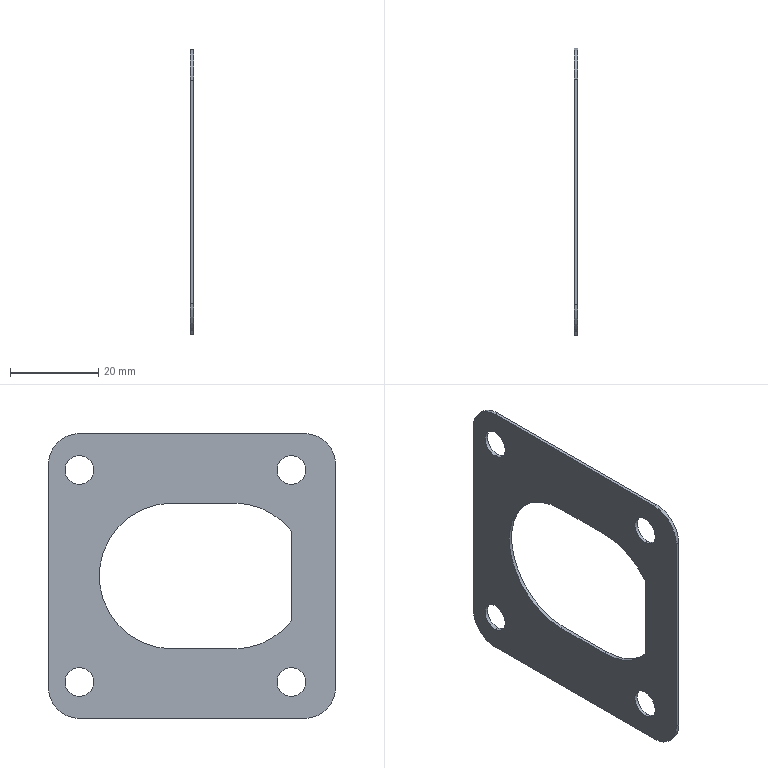Part | SolidWorks | features BaseBody 1 | 1 solid | 24 faces | box 0.8 x 65 x 64.5 mm | volume 2199 mm3 | cylinder 15 | plane 9 | commonest cylinder face diameters 6.5 x8 14 x4 33 x3
STEP:
#1=CARTESIAN_POINT('',(438.9,15.,20.75));
#2=VERTEX_POINT('',#1);
#3=CARTESIAN_POINT('',(438.9,15.,27.25));
#4=VERTEX_POINT('',#3);
#5=CARTESIAN_POINT('',(438.9,15.,24.));
#6=DIRECTION('',(1.,0.,0.));
#7=DIRECTION('',(0.,0.,-1.));
#8=AXIS2_PLACEMENT_3D('',#5,#6,#7);
#9=CIRCLE('',#8,3.25);
#10=EDGE_CURVE('',#2,#4,#9,.T.);
#11=ORIENTED_EDGE('',*,*,#10,.T.);
#12=CARTESIAN_POINT('',(438.1,15.,27.25));
#13=VERTEX_POINT('',#12);
#14=CARTESIAN_POINT('',(438.9,15.,27.25));
#15=DIRECTION('',(-1.,0.,0.));
#16=VECTOR('',#15,1000.);
#17=LINE('',#14,#16);
#18=EDGE_CURVE('',#4,#13,#17,.T.);
#19=ORIENTED_EDGE('',*,*,#18,.T.);
#20=CARTESIAN_POINT('',(438.1,15.,20.75));
#21=VERTEX_POINT('',#20);
#22=CARTESIAN_POINT('',(438.1,15.,24.));
#23=DIRECTION('',(1.,0.,0.));
#24=DIRECTION('',(0.,0.,-1.));
#25=AXIS2_PLACEMENT_3D('',#22,#23,#24);
#26=CIRCLE('',#25,3.25);
#27=EDGE_CURVE('',#21,#13,#26,.T.);
#28=ORIENTED_EDGE('',*,*,#27,.F.);
#29=CARTESIAN_POINT('',(438.9,15.,20.75));
#30=DIRECTION('',(-1.,0.,0.));
#31=VECTOR('',#30,1000.);
#32=LINE('',#29,#31);
#33=EDGE_CURVE('',#2,#21,#32,.T.);
#34=ORIENTED_EDGE('',*,*,#33,.F.);
#35=EDGE_LOOP('',(#11,#19,#28,#34));
#36=FACE_OUTER_BOUND('',#35,.T.);
#37=CARTESIAN_POINT('',(438.9,15.,24.));
#38=DIRECTION('',(-1.,0.,0.));
#39=DIRECTION('',(0.,0.,-1.));
#40=AXIS2_PLACEMENT_3D('',#37,#38,#39);
#41=CYLINDRICAL_SURFACE('',#40,3.25);
#42=ADVANCED_FACE('',(#36),#41,.F.);
#43=CARTESIAN_POINT('',(438.9,63.,20.75));
#44=VERTEX_POINT('',#43);
#45=CARTESIAN_POINT('',(438.9,63.,27.25));
#46=VERTEX_POINT('',#45);
#47=CARTESIAN_POINT('',(438.9,63.,24.));
#48=DIRECTION('',(1.,0.,0.));
#49=DIRECTION('',(0.,0.,-1.));
#50=AXIS2_PLACEMENT_3D('',#47,#48,#49);
#51=CIRCLE('',#50,3.25);
#52=EDGE_CURVE('',#44,#46,#51,.T.);
#53=ORIENTED_EDGE('',*,*,#52,.T.);
#54=CARTESIAN_POINT('',(438.1,63.,27.25));
#55=VERTEX_POINT('',#54);
#56=CARTESIAN_POINT('',(438.9,63.,27.25));
#57=DIRECTION('',(-1.,0.,0.));
#58=VECTOR('',#57,1000.);
#59=LINE('',#56,#58);
#60=EDGE_CURVE('',#46,#55,#59,.T.);
#61=ORIENTED_EDGE('',*,*,#60,.T.);
#62=CARTESIAN_POINT('',(438.1,63.,20.75));
#63=VERTEX_POINT('',#62);
#64=CARTESIAN_POINT('',(438.1,63.,24.));
#65=DIRECTION('',(1.,0.,0.));
#66=DIRECTION('',(0.,0.,-1.));
#67=AXIS2_PLACEMENT_3D('',#64,#65,#66);
#68=CIRCLE('',#67,3.25);
#69=EDGE_CURVE('',#63,#55,#68,.T.);
#70=ORIENTED_EDGE('',*,*,#69,.F.);
#71=CARTESIAN_POINT('',(438.9,63.,20.75));
#72=DIRECTION('',(-1.,0.,0.));
#73=VECTOR('',#72,1000.);
#74=LINE('',#71,#73);
#75=EDGE_CURVE('',#44,#63,#74,.T.);
#76=ORIENTED_EDGE('',*,*,#75,.F.);
#77=EDGE_LOOP('',(#53,#61,#70,#76));
#78=FACE_OUTER_BOUND('',#77,.T.);
#79=CARTESIAN_POINT('',(438.9,63.,24.));
#80=DIRECTION('',(-1.,0.,0.));
#81=DIRECTION('',(0.,0.,-1.));
#82=AXIS2_PLACEMENT_3D('',#79,#80,#81);
#83=CYLINDRICAL_SURFACE('',#82,3.25);
#84=ADVANCED_FACE('',(#78),#83,.F.);
#85=CARTESIAN_POINT('',(438.9,15.,-27.25));
#86=VERTEX_POINT('',#85);
#87=CARTESIAN_POINT('',(438.9,15.,-20.75));
#88=VERTEX_POINT('',#87);
#89=CARTESIAN_POINT('',(438.9,15.,-24.));
#90=DIRECTION('',(1.,0.,0.));
#91=DIRECTION('',(0.,0.,1.));
#92=AXIS2_PLACEMENT_3D('',#89,#90,#91);
#93=CIRCLE('',#92,3.25);
#94=EDGE_CURVE('',#86,#88,#93,.T.);
#95=ORIENTED_EDGE('',*,*,#94,.T.);
#96=CARTESIAN_POINT('',(438.1,15.,-20.75));
#97=VERTEX_POINT('',#96);
#98=CARTESIAN_POINT('',(438.9,15.,-20.75));
#99=DIRECTION('',(-1.,0.,0.));
#100=VECTOR('',#99,1000.);
#101=LINE('',#98,#100);
#102=EDGE_CURVE('',#88,#97,#101,.T.);
#103=ORIENTED_EDGE('',*,*,#102,.T.);
#104=CARTESIAN_POINT('',(438.1,15.,-27.25));
#105=VERTEX_POINT('',#104);
#106=CARTESIAN_POINT('',(438.1,15.,-24.));
#107=DIRECTION('',(1.,0.,0.));
#108=DIRECTION('',(0.,0.,1.));
#109=AXIS2_PLACEMENT_3D('',#106,#107,#108);
#110=CIRCLE('',#109,3.25);
#111=EDGE_CURVE('',#105,#97,#110,.T.);
#112=ORIENTED_EDGE('',*,*,#111,.F.);
#113=CARTESIAN_POINT('',(438.9,15.,-27.25));
#114=DIRECTION('',(-1.,0.,0.));
#115=VECTOR('',#114,1000.);
#116=LINE('',#113,#115);
#117=EDGE_CURVE('',#86,#105,#116,.T.);
#118=ORIENTED_EDGE('',*,*,#117,.F.);
#119=EDGE_LOOP('',(#95,#103,#112,#118));
#120=FACE_OUTER_BOUND('',#119,.T.);
#121=CARTESIAN_POINT('',(438.9,15.,-24.));
#122=DIRECTION('',(-1.,0.,0.));
#123=DIRECTION('',(0.,0.,-1.));
#124=AXIS2_PLACEMENT_3D('',#121,#122,#123);
#125=CYLINDRICAL_SURFACE('',#124,3.25);
#126=ADVANCED_FACE('',(#120),#125,.F.);
#127=CARTESIAN_POINT('',(438.9,63.,-27.25));
#128=VERTEX_POINT('',#127);
#129=CARTESIAN_POINT('',(438.9,63.,-20.75));
#130=VERTEX_POINT('',#129);
#131=CARTESIAN_POINT('',(438.9,63.,-24.));
#132=DIRECTION('',(1.,0.,0.));
#133=DIRECTION('',(0.,0.,1.));
#134=AXIS2_PLACEMENT_3D('',#131,#132,#133);
#135=CIRCLE('',#134,3.25);
#136=EDGE_CURVE('',#128,#130,#135,.T.);
#137=ORIENTED_EDGE('',*,*,#136,.T.);
#138=CARTESIAN_POINT('',(438.1,63.,-20.75));
#139=VERTEX_POINT('',#138);
#140=CARTESIAN_POINT('',(438.9,63.,-20.75));
#141=DIRECTION('',(-1.,0.,0.));
#142=VECTOR('',#141,1000.);
#143=LINE('',#140,#142);
#144=EDGE_CURVE('',#130,#139,#143,.T.);
#145=ORIENTED_EDGE('',*,*,#144,.T.);
#146=CARTESIAN_POINT('',(438.1,63.,-27.25));
#147=VERTEX_POINT('',#146);
#148=CARTESIAN_POINT('',(438.1,63.,-24.));
#149=DIRECTION('',(1.,0.,0.));
#150=DIRECTION('',(0.,0.,1.));
#151=AXIS2_PLACEMENT_3D('',#148,#149,#150);
#152=CIRCLE('',#151,3.25);
#153=EDGE_CURVE('',#147,#139,#152,.T.);
#154=ORIENTED_EDGE('',*,*,#153,.F.);
#155=CARTESIAN_POINT('',(438.9,63.,-27.25));
#156=DIRECTION('',(-1.,0.,0.));
#157=VECTOR('',#156,1000.);
#158=LINE('',#155,#157);
#159=EDGE_CURVE('',#128,#147,#158,.T.);
#160=ORIENTED_EDGE('',*,*,#159,.F.);
#161=EDGE_LOOP('',(#137,#145,#154,#160));
#162=FACE_OUTER_BOUND('',#161,.T.);
#163=CARTESIAN_POINT('',(438.9,63.,-24.));
#164=DIRECTION('',(-1.,0.,0.));
#165=DIRECTION('',(0.,0.,-1.));
#166=AXIS2_PLACEMENT_3D('',#163,#164,#165);
#167=CYLINDRICAL_SURFACE('',#166,3.25);
#168=ADVANCED_FACE('',(#162),#167,.F.);
#169=ORIENTED_EDGE('',*,*,#52,.F.);
#170=CARTESIAN_POINT('',(438.9,63.,24.));
#171=DIRECTION('',(1.,0.,0.));
#172=DIRECTION('',(0.,0.,-1.));
#173=AXIS2_PLACEMENT_3D('',#170,#171,#172);
#174=CIRCLE('',#173,3.25);
#175=EDGE_CURVE('',#46,#44,#174,.T.);
#176=ORIENTED_EDGE('',*,*,#175,.F.);
#177=EDGE_LOOP('',(#169,#176));
#178=FACE_BOUND('',#177,.T.);
#179=ORIENTED_EDGE('',*,*,#94,.F.);
#180=CARTESIAN_POINT('',(438.9,15.,-24.));
#181=DIRECTION('',(1.,0.,0.));
#182=DIRECTION('',(0.,0.,1.));
#183=AXIS2_PLACEMENT_3D('',#180,#181,#182);
#184=CIRCLE('',#183,3.25);
#185=EDGE_CURVE('',#88,#86,#184,.T.);
#186=ORIENTED_EDGE('',*,*,#185,.F.);
#187=EDGE_LOOP('',(#179,#186));
#188=FACE_BOUND('',#187,.T.);
#189=CARTESIAN_POINT('',(438.9,5.,-25.25));
#190=VERTEX_POINT('',#189);
#191=CARTESIAN_POINT('',(438.9,12.,-32.25));
#192=VERTEX_POINT('',#191);
#193=CARTESIAN_POINT('',(438.9,12.,-25.25));
#194=DIRECTION('',(1.,0.,0.));
#195=DIRECTION('',(0.,0.,1.));
#196=AXIS2_PLACEMENT_3D('',#193,#194,#195);
#197=CIRCLE('',#196,7.);
#198=EDGE_CURVE('',#190,#192,#197,.T.);
#199=ORIENTED_EDGE('',*,*,#198,.T.);
#200=CARTESIAN_POINT('',(438.9,63.,-32.25));
#201=VERTEX_POINT('',#200);
#202=CARTESIAN_POINT('',(438.9,12.,-32.25));
#203=DIRECTION('',(0.,1.,0.));
#204=VECTOR('',#203,1000.);
#205=LINE('',#202,#204);
#206=EDGE_CURVE('',#192,#201,#205,.T.);
#207=ORIENTED_EDGE('',*,*,#206,.T.);
#208=CARTESIAN_POINT('',(438.9,70.,-25.25));
#209=VERTEX_POINT('',#208);
#210=CARTESIAN_POINT('',(438.9,63.,-25.25));
#211=DIRECTION('',(1.,0.,0.));
#212=DIRECTION('',(0.,0.,1.));
#213=AXIS2_PLACEMENT_3D('',#210,#211,#212);
#214=CIRCLE('',#213,7.);
#215=EDGE_CURVE('',#201,#209,#214,.T.);
#216=ORIENTED_EDGE('',*,*,#215,.T.);
#217=CARTESIAN_POINT('',(438.9,70.,25.25));
#218=VERTEX_POINT('',#217);
#219=CARTESIAN_POINT('',(438.9,70.,-25.25));
#220=DIRECTION('',(0.,0.,1.));
#221=VECTOR('',#220,1000.);
#222=LINE('',#219,#221);
#223=EDGE_CURVE('',#209,#218,#222,.T.);
#224=ORIENTED_EDGE('',*,*,#223,.T.);
#225=CARTESIAN_POINT('',(438.9,63.,32.25));
#226=VERTEX_POINT('',#225);
#227=CARTESIAN_POINT('',(438.9,63.,25.25));
#228=DIRECTION('',(1.,0.,0.));
#229=DIRECTION('',(0.,0.,1.));
#230=AXIS2_PLACEMENT_3D('',#227,#228,#229);
#231=CIRCLE('',#230,7.);
#232=EDGE_CURVE('',#218,#226,#231,.T.);
#233=ORIENTED_EDGE('',*,*,#232,.T.);
#234=CARTESIAN_POINT('',(438.9,12.,32.25));
#235=VERTEX_POINT('',#234);
#236=CARTESIAN_POINT('',(438.9,12.,32.25));
#237=DIRECTION('',(0.,-1.,0.));
#238=VECTOR('',#237,1000.);
#239=LINE('',#236,#238);
#240=EDGE_CURVE('',#226,#235,#239,.T.);
#241=ORIENTED_EDGE('',*,*,#240,.T.);
#242=CARTESIAN_POINT('',(438.9,5.,25.25));
#243=VERTEX_POINT('',#242);
#244=CARTESIAN_POINT('',(438.9,12.,25.25));
#245=DIRECTION('',(1.,0.,0.));
#246=DIRECTION('',(0.,0.,-1.));
#247=AXIS2_PLACEMENT_3D('',#244,#245,#246);
#248=CIRCLE('',#247,7.);
#249=EDGE_CURVE('',#235,#243,#248,.T.);
#250=ORIENTED_EDGE('',*,*,#249,.T.);
#251=CARTESIAN_POINT('',(438.9,5.,-25.25));
#252=DIRECTION('',(0.,0.,-1.));
#253=VECTOR('',#252,1000.);
#254=LINE('',#251,#253);
#255=EDGE_CURVE('',#243,#190,#254,.T.);
#256=ORIENTED_EDGE('',*,*,#255,.T.);
#257=EDGE_LOOP('',(#199,#207,#216,#224,#233,#241,#250,#256));
#258=FACE_OUTER_BOUND('',#257,.T.);
#259=ORIENTED_EDGE('',*,*,#136,.F.);
#260=CARTESIAN_POINT('',(438.9,63.,-24.));
#261=DIRECTION('',(1.,0.,0.));
#262=DIRECTION('',(0.,0.,1.));
#263=AXIS2_PLACEMENT_3D('',#260,#261,#262);
#264=CIRCLE('',#263,3.25);
#265=EDGE_CURVE('',#130,#128,#264,.T.);
#266=ORIENTED_EDGE('',*,*,#265,.F.);
#267=EDGE_LOOP('',(#259,#266));
#268=FACE_BOUND('',#267,.T.);
#269=CARTESIAN_POINT('',(438.9,15.,10.161));
#270=VERTEX_POINT('',#269);
#271=CARTESIAN_POINT('',(438.9,15.,-10.161));
#272=VERTEX_POINT('',#271);
#273=CARTESIAN_POINT('',(438.9,15.,-10.161));
#274=DIRECTION('',(0.,0.,-1.));
#275=VECTOR('',#274,1000.);
#276=LINE('',#273,#275);
#277=EDGE_CURVE('',#270,#272,#276,.T.);
#278=ORIENTED_EDGE('',*,*,#277,.F.);
#279=CARTESIAN_POINT('',(438.9,28.,16.5));
#280=VERTEX_POINT('',#279);
#281=CARTESIAN_POINT('',(438.9,28.,0.));
#282=DIRECTION('',(1.,0.,0.));
#283=DIRECTION('',(0.,0.,1.));
#284=AXIS2_PLACEMENT_3D('',#281,#282,#283);
#285=CIRCLE('',#284,16.5);
#286=EDGE_CURVE('',#280,#270,#285,.T.);
#287=ORIENTED_EDGE('',*,*,#286,.F.);
#288=CARTESIAN_POINT('',(438.9,42.,16.5));
#289=VERTEX_POINT('',#288);
#290=CARTESIAN_POINT('',(438.9,28.,16.5));
#291=DIRECTION('',(0.,-1.,0.));
#292=VECTOR('',#291,1000.);
#293=LINE('',#290,#292);
#294=EDGE_CURVE('',#289,#280,#293,.T.);
#295=ORIENTED_EDGE('',*,*,#294,.F.);
#296=CARTESIAN_POINT('',(438.9,42.,-16.5));
#297=VERTEX_POINT('',#296);
#298=CARTESIAN_POINT('',(438.9,42.,0.));
#299=DIRECTION('',(1.,0.,0.));
#300=DIRECTION('',(0.,0.,1.));
#301=AXIS2_PLACEMENT_3D('',#298,#299,#300);
#302=CIRCLE('',#301,16.5);
#303=EDGE_CURVE('',#297,#289,#302,.T.);
#304=ORIENTED_EDGE('',*,*,#303,.F.);
#305=CARTESIAN_POINT('',(438.9,28.,-16.5));
#306=VERTEX_POINT('',#305);
#307=CARTESIAN_POINT('',(438.9,42.,-16.5));
#308=DIRECTION('',(0.,1.,0.));
#309=VECTOR('',#308,1000.);
#310=LINE('',#307,#309);
#311=EDGE_CURVE('',#306,#297,#310,.T.);
#312=ORIENTED_EDGE('',*,*,#311,.F.);
#313=CARTESIAN_POINT('',(438.9,28.,0.));
#314=DIRECTION('',(1.,0.,0.));
#315=DIRECTION('',(0.,0.,1.));
#316=AXIS2_PLACEMENT_3D('',#313,#314,#315);
#317=CIRCLE('',#316,16.5);
#318=EDGE_CURVE('',#272,#306,#317,.T.);
#319=ORIENTED_EDGE('',*,*,#318,.F.);
#320=EDGE_LOOP('',(#278,#287,#295,#304,#312,#319));
#321=FACE_BOUND('',#320,.T.);
#322=ORIENTED_EDGE('',*,*,#10,.F.);
#323=CARTESIAN_POINT('',(438.9,15.,24.));
#324=DIRECTION('',(1.,0.,0.));
#325=DIRECTION('',(0.,0.,-1.));
#326=AXIS2_PLACEMENT_3D('',#323,#324,#325);
#327=CIRCLE('',#326,3.25);
#328=EDGE_CURVE('',#4,#2,#327,.T.);
#329=ORIENTED_EDGE('',*,*,#328,.F.);
#330=EDGE_LOOP('',(#322,#329));
#331=FACE_BOUND('',#330,.T.);
#332=CARTESIAN_POINT('',(438.9,12.,-25.25));
#333=DIRECTION('',(1.,0.,0.));
#334=DIRECTION('',(0.,0.,1.));
#335=AXIS2_PLACEMENT_3D('',#332,#333,#334);
#336=PLANE('',#335);
#337=ADVANCED_FACE('',(#178,#188,#258,#268,#321,#331),#336,.T.);
#338=ORIENTED_EDGE('',*,*,#69,.T.);
#339=CARTESIAN_POINT('',(438.1,63.,24.));
#340=DIRECTION('',(1.,0.,0.));
#341=DIRECTION('',(0.,0.,-1.));
#342=AXIS2_PLACEMENT_3D('',#339,#340,#341);
#343=CIRCLE('',#342,3.25);
#344=EDGE_CURVE('',#55,#63,#343,.T.);
#345=ORIENTED_EDGE('',*,*,#344,.T.);
#346=EDGE_LOOP('',(#338,#345));
#347=FACE_BOUND('',#346,.T.);
#348=ORIENTED_EDGE('',*,*,#111,.T.);
#349=CARTESIAN_POINT('',(438.1,15.,-24.));
#350=DIRECTION('',(1.,0.,0.));
#351=DIRECTION('',(0.,0.,1.));
#352=AXIS2_PLACEMENT_3D('',#349,#350,#351);
#353=CIRCLE('',#352,3.25);
#354=EDGE_CURVE('',#97,#105,#353,.T.);
#355=ORIENTED_EDGE('',*,*,#354,.T.);
#356=EDGE_LOOP('',(#348,#355));
#357=FACE_BOUND('',#356,.T.);
#358=CARTESIAN_POINT('',(438.1,5.,-25.25));
#359=VERTEX_POINT('',#358);
#360=CARTESIAN_POINT('',(438.1,12.,-32.25));
#361=VERTEX_POINT('',#360);
#362=CARTESIAN_POINT('',(438.1,12.,-25.25));
#363=DIRECTION('',(1.,0.,0.));
#364=DIRECTION('',(0.,0.,1.));
#365=AXIS2_PLACEMENT_3D('',#362,#363,#364);
#366=CIRCLE('',#365,7.);
#367=EDGE_CURVE('',#359,#361,#366,.T.);
#368=ORIENTED_EDGE('',*,*,#367,.F.);
#369=CARTESIAN_POINT('',(438.1,5.,25.25));
#370=VERTEX_POINT('',#369);
#371=CARTESIAN_POINT('',(438.1,5.,-25.25));
#372=DIRECTION('',(0.,0.,-1.));
#373=VECTOR('',#372,1000.);
#374=LINE('',#371,#373);
#375=EDGE_CURVE('',#370,#359,#374,.T.);
#376=ORIENTED_EDGE('',*,*,#375,.F.);
#377=CARTESIAN_POINT('',(438.1,12.,32.25));
#378=VERTEX_POINT('',#377);
#379=CARTESIAN_POINT('',(438.1,12.,25.25));
#380=DIRECTION('',(1.,0.,0.));
#381=DIRECTION('',(0.,0.,-1.));
#382=AXIS2_PLACEMENT_3D('',#379,#380,#381);
#383=CIRCLE('',#382,7.);
#384=EDGE_CURVE('',#378,#370,#383,.T.);
#385=ORIENTED_EDGE('',*,*,#384,.F.);
#386=CARTESIAN_POINT('',(438.1,63.,32.25));
#387=VERTEX_POINT('',#386);
#388=CARTESIAN_POINT('',(438.1,12.,32.25));
#389=DIRECTION('',(0.,-1.,0.));
#390=VECTOR('',#389,1000.);
#391=LINE('',#388,#390);
#392=EDGE_CURVE('',#387,#378,#391,.T.);
#393=ORIENTED_EDGE('',*,*,#392,.F.);
#394=CARTESIAN_POINT('',(438.1,70.,25.25));
#395=VERTEX_POINT('',#394);
#396=CARTESIAN_POINT('',(438.1,63.,25.25));
#397=DIRECTION('',(1.,0.,0.));
#398=DIRECTION('',(0.,0.,1.));
#399=AXIS2_PLACEMENT_3D('',#396,#397,#398);
#400=CIRCLE('',#399,7.);
#401=EDGE_CURVE('',#395,#387,#400,.T.);
#402=ORIENTED_EDGE('',*,*,#401,.F.);
#403=CARTESIAN_POINT('',(438.1,70.,-25.25));
#404=VERTEX_POINT('',#403);
#405=CARTESIAN_POINT('',(438.1,70.,-25.25));
#406=DIRECTION('',(0.,0.,1.));
#407=VECTOR('',#406,1000.);
#408=LINE('',#405,#407);
#409=EDGE_CURVE('',#404,#395,#408,.T.);
#410=ORIENTED_EDGE('',*,*,#409,.F.);
#411=CARTESIAN_POINT('',(438.1,63.,-32.25));
#412=VERTEX_POINT('',#411);
#413=CARTESIAN_POINT('',(438.1,63.,-25.25));
#414=DIRECTION('',(1.,0.,0.));
#415=DIRECTION('',(0.,0.,1.));
#416=AXIS2_PLACEMENT_3D('',#413,#414,#415);
#417=CIRCLE('',#416,7.);
#418=EDGE_CURVE('',#412,#404,#417,.T.);
#419=ORIENTED_EDGE('',*,*,#418,.F.);
#420=CARTESIAN_POINT('',(438.1,12.,-32.25));
#421=DIRECTION('',(0.,1.,0.));
#422=VECTOR('',#421,1000.);
#423=LINE('',#420,#422);
#424=EDGE_CURVE('',#361,#412,#423,.T.);
#425=ORIENTED_EDGE('',*,*,#424,.F.);
#426=EDGE_LOOP('',(#368,#376,#385,#393,#402,#410,#419,#425));
#427=FACE_OUTER_BOUND('',#426,.T.);
#428=ORIENTED_EDGE('',*,*,#153,.T.);
#429=CARTESIAN_POINT('',(438.1,63.,-24.));
#430=DIRECTION('',(1.,0.,0.));
#431=DIRECTION('',(0.,0.,1.));
#432=AXIS2_PLACEMENT_3D('',#429,#430,#431);
#433=CIRCLE('',#432,3.25);
#434=EDGE_CURVE('',#139,#147,#433,.T.);
#435=ORIENTED_EDGE('',*,*,#434,.T.);
#436=EDGE_LOOP('',(#428,#435));
#437=FACE_BOUND('',#436,.T.);
#438=CARTESIAN_POINT('',(438.1,28.,16.5));
#439=VERTEX_POINT('',#438);
#440=CARTESIAN_POINT('',(438.1,15.,10.161));
#441=VERTEX_POINT('',#440);
#442=CARTESIAN_POINT('',(438.1,28.,0.));
#443=DIRECTION('',(1.,0.,0.));
#444=DIRECTION('',(0.,0.,1.));
#445=AXIS2_PLACEMENT_3D('',#442,#443,#444);
#446=CIRCLE('',#445,16.5);
#447=EDGE_CURVE('',#439,#441,#446,.T.);
#448=ORIENTED_EDGE('',*,*,#447,.T.);
#449=CARTESIAN_POINT('',(438.1,15.,-10.161));
#450=VERTEX_POINT('',#449);
#451=CARTESIAN_POINT('',(438.1,15.,-10.161));
#452=DIRECTION('',(0.,0.,-1.));
#453=VECTOR('',#452,1000.);
#454=LINE('',#451,#453);
#455=EDGE_CURVE('',#441,#450,#454,.T.);
#456=ORIENTED_EDGE('',*,*,#455,.T.);
#457=CARTESIAN_POINT('',(438.1,28.,-16.5));
#458=VERTEX_POINT('',#457);
#459=CARTESIAN_POINT('',(438.1,28.,0.));
#460=DIRECTION('',(1.,0.,0.));
#461=DIRECTION('',(0.,0.,1.));
#462=AXIS2_PLACEMENT_3D('',#459,#460,#461);
#463=CIRCLE('',#462,16.5);
#464=EDGE_CURVE('',#450,#458,#463,.T.);
#465=ORIENTED_EDGE('',*,*,#464,.T.);
#466=CARTESIAN_POINT('',(438.1,42.,-16.5));
#467=VERTEX_POINT('',#466);
#468=CARTESIAN_POINT('',(438.1,42.,-16.5));
#469=DIRECTION('',(0.,1.,0.));
#470=VECTOR('',#469,1000.);
#471=LINE('',#468,#470);
#472=EDGE_CURVE('',#458,#467,#471,.T.);
#473=ORIENTED_EDGE('',*,*,#472,.T.);
#474=CARTESIAN_POINT('',(438.1,42.,16.5));
#475=VERTEX_POINT('',#474);
#476=CARTESIAN_POINT('',(438.1,42.,0.));
#477=DIRECTION('',(1.,0.,0.));
#478=DIRECTION('',(0.,0.,1.));
#479=AXIS2_PLACEMENT_3D('',#476,#477,#478);
#480=CIRCLE('',#479,16.5);
#481=EDGE_CURVE('',#467,#475,#480,.T.);
#482=ORIENTED_EDGE('',*,*,#481,.T.);
#483=CARTESIAN_POINT('',(438.1,28.,16.5));
#484=DIRECTION('',(0.,-1.,0.));
#485=VECTOR('',#484,1000.);
#486=LINE('',#483,#485);
#487=EDGE_CURVE('',#475,#439,#486,.T.);
#488=ORIENTED_EDGE('',*,*,#487,.T.);
#489=EDGE_LOOP('',(#448,#456,#465,#473,#482,#488));
#490=FACE_BOUND('',#489,.T.);
#491=ORIENTED_EDGE('',*,*,#27,.T.);
#492=CARTESIAN_POINT('',(438.1,15.,24.));
#493=DIRECTION('',(1.,0.,0.));
#494=DIRECTION('',(0.,0.,-1.));
#495=AXIS2_PLACEMENT_3D('',#492,#493,#494);
#496=CIRCLE('',#495,3.25);
#497=EDGE_CURVE('',#13,#21,#496,.T.);
#498=ORIENTED_EDGE('',*,*,#497,.T.);
#499=EDGE_LOOP('',(#491,#498));
#500=FACE_BOUND('',#499,.T.);
#501=CARTESIAN_POINT('',(438.1,12.,-25.25));
#502=DIRECTION('',(1.,0.,0.));
#503=DIRECTION('',(0.,0.,1.));
#504=AXIS2_PLACEMENT_3D('',#501,#502,#503);
#505=PLANE('',#504);
#506=ADVANCED_FACE('',(#347,#357,#427,#437,#490,#500),#505,.F.);
#507=ORIENTED_EDGE('',*,*,#367,.T.);
#508=CARTESIAN_POINT('',(438.9,12.,-32.25));
#509=DIRECTION('',(-1.,0.,0.));
#510=VECTOR('',#509,1000.);
#511=LINE('',#508,#510);
#512=EDGE_CURVE('',#192,#361,#511,.T.);
#513=ORIENTED_EDGE('',*,*,#512,.F.);
#514=ORIENTED_EDGE('',*,*,#198,.F.);
#515=CARTESIAN_POINT('',(438.9,5.,-25.25));
#516=DIRECTION('',(-1.,0.,0.));
#517=VECTOR('',#516,1000.);
#518=LINE('',#515,#517);
#519=EDGE_CURVE('',#190,#359,#518,.T.);
#520=ORIENTED_EDGE('',*,*,#519,.T.);
#521=EDGE_LOOP('',(#507,#513,#514,#520));
#522=FACE_OUTER_BOUND('',#521,.T.);
#523=CARTESIAN_POINT('',(438.9,12.,-25.25));
#524=DIRECTION('',(-1.,0.,0.));
#525=DIRECTION('',(0.,0.,-1.));
#526=AXIS2_PLACEMENT_3D('',#523,#524,#525);
#527=CYLINDRICAL_SURFACE('',#526,7.);
#528=ADVANCED_FACE('',(#522),#527,.T.);
#529=ORIENTED_EDGE('',*,*,#424,.T.);
#530=CARTESIAN_POINT('',(438.9,63.,-32.25));
#531=DIRECTION('',(-1.,0.,0.));
#532=VECTOR('',#531,1000.);
#533=LINE('',#530,#532);
#534=EDGE_CURVE('',#201,#412,#533,.T.);
#535=ORIENTED_EDGE('',*,*,#534,.F.);
#536=ORIENTED_EDGE('',*,*,#206,.F.);
#537=ORIENTED_EDGE('',*,*,#512,.T.);
#538=EDGE_LOOP('',(#529,#535,#536,#537));
#539=FACE_OUTER_BOUND('',#538,.T.);
#540=CARTESIAN_POINT('',(438.9,12.,-32.25));
#541=DIRECTION('',(0.,0.,1.));
#542=DIRECTION('',(-1.,0.,0.));
#543=AXIS2_PLACEMENT_3D('',#540,#541,#542);
#544=PLANE('',#543);
#545=ADVANCED_FACE('',(#539),#544,.F.);
#546=ORIENTED_EDGE('',*,*,#418,.T.);
#547=CARTESIAN_POINT('',(438.9,70.,-25.25));
#548=DIRECTION('',(-1.,0.,0.));
#549=VECTOR('',#548,1000.);
#550=LINE('',#547,#549);
#551=EDGE_CURVE('',#209,#404,#550,.T.);
#552=ORIENTED_EDGE('',*,*,#551,.F.);
#553=ORIENTED_EDGE('',*,*,#215,.F.);
#554=ORIENTED_EDGE('',*,*,#534,.T.);
#555=EDGE_LOOP('',(#546,#552,#553,#554));
#556=FACE_OUTER_BOUND('',#555,.T.);
#557=CARTESIAN_POINT('',(438.9,63.,-25.25));
#558=DIRECTION('',(-1.,0.,0.));
#559=DIRECTION('',(0.,0.,-1.));
#560=AXIS2_PLACEMENT_3D('',#557,#558,#559);
#561=CYLINDRICAL_SURFACE('',#560,7.);
#562=ADVANCED_FACE('',(#556),#561,.T.);
#563=ORIENTED_EDGE('',*,*,#409,.T.);
#564=CARTESIAN_POINT('',(438.9,70.,25.25));
#565=DIRECTION('',(-1.,0.,0.));
#566=VECTOR('',#565,1000.);
#567=LINE('',#564,#566);
#568=EDGE_CURVE('',#218,#395,#567,.T.);
#569=ORIENTED_EDGE('',*,*,#568,.F.);
#570=ORIENTED_EDGE('',*,*,#223,.F.);
#571=ORIENTED_EDGE('',*,*,#551,.T.);
#572=EDGE_LOOP('',(#563,#569,#570,#571));
#573=FACE_OUTER_BOUND('',#572,.T.);
#574=CARTESIAN_POINT('',(438.9,70.,-25.25));
#575=DIRECTION('',(0.,-1.,0.));
#576=DIRECTION('',(0.,0.,-1.));
#577=AXIS2_PLACEMENT_3D('',#574,#575,#576);
#578=PLANE('',#577);
#579=ADVANCED_FACE('',(#573),#578,.F.);
#580=ORIENTED_EDGE('',*,*,#401,.T.);
#581=CARTESIAN_POINT('',(438.9,63.,32.25));
#582=DIRECTION('',(-1.,0.,0.));
#583=VECTOR('',#582,1000.);
#584=LINE('',#581,#583);
#585=EDGE_CURVE('',#226,#387,#584,.T.);
#586=ORIENTED_EDGE('',*,*,#585,.F.);
#587=ORIENTED_EDGE('',*,*,#232,.F.);
#588=ORIENTED_EDGE('',*,*,#568,.T.);
#589=EDGE_LOOP('',(#580,#586,#587,#588));
#590=FACE_OUTER_BOUND('',#589,.T.);
#591=CARTESIAN_POINT('',(438.9,63.,25.25));
#592=DIRECTION('',(-1.,0.,0.));
#593=DIRECTION('',(0.,0.,-1.));
#594=AXIS2_PLACEMENT_3D('',#591,#592,#593);
#595=CYLINDRICAL_SURFACE('',#594,7.);
#596=ADVANCED_FACE('',(#590),#595,.T.);
#597=ORIENTED_EDGE('',*,*,#392,.T.);
#598=CARTESIAN_POINT('',(438.9,12.,32.25));
#599=DIRECTION('',(-1.,0.,0.));
#600=VECTOR('',#599,1000.);
#601=LINE('',#598,#600);
#602=EDGE_CURVE('',#235,#378,#601,.T.);
#603=ORIENTED_EDGE('',*,*,#602,.F.);
#604=ORIENTED_EDGE('',*,*,#240,.F.);
#605=ORIENTED_EDGE('',*,*,#585,.T.);
#606=EDGE_LOOP('',(#597,#603,#604,#605));
#607=FACE_OUTER_BOUND('',#606,.T.);
#608=CARTESIAN_POINT('',(438.9,12.,32.25));
#609=DIRECTION('',(0.,0.,-1.));
#610=DIRECTION('',(0.,1.,0.));
#611=AXIS2_PLACEMENT_3D('',#608,#609,#610);
#612=PLANE('',#611);
#613=ADVANCED_FACE('',(#607),#612,.F.);
#614=ORIENTED_EDGE('',*,*,#384,.T.);
#615=CARTESIAN_POINT('',(438.9,5.,25.25));
#616=DIRECTION('',(-1.,0.,0.));
#617=VECTOR('',#616,1000.);
#618=LINE('',#615,#617);
#619=EDGE_CURVE('',#243,#370,#618,.T.);
#620=ORIENTED_EDGE('',*,*,#619,.F.);
#621=ORIENTED_EDGE('',*,*,#249,.F.);
#622=ORIENTED_EDGE('',*,*,#602,.T.);
#623=EDGE_LOOP('',(#614,#620,#621,#622));
#624=FACE_OUTER_BOUND('',#623,.T.);
#625=CARTESIAN_POINT('',(438.9,12.,25.25));
#626=DIRECTION('',(-1.,0.,0.));
#627=DIRECTION('',(0.,0.,-1.));
#628=AXIS2_PLACEMENT_3D('',#625,#626,#627);
#629=CYLINDRICAL_SURFACE('',#628,7.);
#630=ADVANCED_FACE('',(#624),#629,.T.);
#631=ORIENTED_EDGE('',*,*,#375,.T.);
#632=ORIENTED_EDGE('',*,*,#519,.F.);
#633=ORIENTED_EDGE('',*,*,#255,.F.);
#634=ORIENTED_EDGE('',*,*,#619,.T.);
#635=EDGE_LOOP('',(#631,#632,#633,#634));
#636=FACE_OUTER_BOUND('',#635,.T.);
#637=CARTESIAN_POINT('',(438.9,5.,-25.25));
#638=DIRECTION('',(0.,1.,0.));
#639=DIRECTION('',(0.,0.,1.));
#640=AXIS2_PLACEMENT_3D('',#637,#638,#639);
#641=PLANE('',#640);
#642=ADVANCED_FACE('',(#636),#641,.F.);
#643=ORIENTED_EDGE('',*,*,#144,.F.);
#644=ORIENTED_EDGE('',*,*,#265,.T.);
#645=ORIENTED_EDGE('',*,*,#159,.T.);
#646=ORIENTED_EDGE('',*,*,#434,.F.);
#647=EDGE_LOOP('',(#643,#644,#645,#646));
#648=FACE_OUTER_BOUND('',#647,.T.);
#649=CARTESIAN_POINT('',(438.9,63.,-24.));
#650=DIRECTION('',(-1.,0.,0.));
#651=DIRECTION('',(0.,0.,-1.));
#652=AXIS2_PLACEMENT_3D('',#649,#650,#651);
#653=CYLINDRICAL_SURFACE('',#652,3.25);
#654=ADVANCED_FACE('',(#648),#653,.F.);
#655=ORIENTED_EDGE('',*,*,#102,.F.);
#656=ORIENTED_EDGE('',*,*,#185,.T.);
#657=ORIENTED_EDGE('',*,*,#117,.T.);
#658=ORIENTED_EDGE('',*,*,#354,.F.);
#659=EDGE_LOOP('',(#655,#656,#657,#658));
#660=FACE_OUTER_BOUND('',#659,.T.);
#661=CARTESIAN_POINT('',(438.9,15.,-24.));
#662=DIRECTION('',(-1.,0.,0.));
#663=DIRECTION('',(0.,0.,-1.));
#664=AXIS2_PLACEMENT_3D('',#661,#662,#663);
#665=CYLINDRICAL_SURFACE('',#664,3.25);
#666=ADVANCED_FACE('',(#660),#665,.F.);
#667=ORIENTED_EDGE('',*,*,#447,.F.);
#668=CARTESIAN_POINT('',(438.9,28.,16.5));
#669=DIRECTION('',(-1.,0.,0.));
#670=VECTOR('',#669,1000.);
#671=LINE('',#668,#670);
#672=EDGE_CURVE('',#280,#439,#671,.T.);
#673=ORIENTED_EDGE('',*,*,#672,.F.);
#674=ORIENTED_EDGE('',*,*,#286,.T.);
#675=CARTESIAN_POINT('',(438.9,15.,10.161));
#676=DIRECTION('',(-1.,0.,0.));
#677=VECTOR('',#676,1000.);
#678=LINE('',#675,#677);
#679=EDGE_CURVE('',#270,#441,#678,.T.);
#680=ORIENTED_EDGE('',*,*,#679,.T.);
#681=EDGE_LOOP('',(#667,#673,#674,#680));
#682=FACE_OUTER_BOUND('',#681,.T.);
#683=CARTESIAN_POINT('',(438.9,28.,0.));
#684=DIRECTION('',(-1.,0.,0.));
#685=DIRECTION('',(0.,0.,-1.));
#686=AXIS2_PLACEMENT_3D('',#683,#684,#685);
#687=CYLINDRICAL_SURFACE('',#686,16.5);
#688=ADVANCED_FACE('',(#682),#687,.F.);
#689=ORIENTED_EDGE('',*,*,#455,.F.);
#690=ORIENTED_EDGE('',*,*,#679,.F.);
#691=ORIENTED_EDGE('',*,*,#277,.T.);
#692=CARTESIAN_POINT('',(438.9,15.,-10.161));
#693=DIRECTION('',(-1.,0.,0.));
#694=VECTOR('',#693,1000.);
#695=LINE('',#692,#694);
#696=EDGE_CURVE('',#272,#450,#695,.T.);
#697=ORIENTED_EDGE('',*,*,#696,.T.);
#698=EDGE_LOOP('',(#689,#690,#691,#697));
#699=FACE_OUTER_BOUND('',#698,.T.);
#700=CARTESIAN_POINT('',(438.9,15.,-10.161));
#701=DIRECTION('',(0.,1.,0.));
#702=DIRECTION('',(-1.,0.,0.));
#703=AXIS2_PLACEMENT_3D('',#700,#701,#702);
#704=PLANE('',#703);
#705=ADVANCED_FACE('',(#699),#704,.T.);
#706=ORIENTED_EDGE('',*,*,#464,.F.);
#707=ORIENTED_EDGE('',*,*,#696,.F.);
#708=ORIENTED_EDGE('',*,*,#318,.T.);
#709=CARTESIAN_POINT('',(438.9,28.,-16.5));
#710=DIRECTION('',(-1.,0.,0.));
#711=VECTOR('',#710,1000.);
#712=LINE('',#709,#711);
#713=EDGE_CURVE('',#306,#458,#712,.T.);
#714=ORIENTED_EDGE('',*,*,#713,.T.);
#715=EDGE_LOOP('',(#706,#707,#708,#714));
#716=FACE_OUTER_BOUND('',#715,.T.);
#717=CARTESIAN_POINT('',(438.9,28.,0.));
#718=DIRECTION('',(-1.,0.,0.));
#719=DIRECTION('',(0.,0.,-1.));
#720=AXIS2_PLACEMENT_3D('',#717,#718,#719);
#721=CYLINDRICAL_SURFACE('',#720,16.5);
#722=ADVANCED_FACE('',(#716),#721,.F.);
#723=ORIENTED_EDGE('',*,*,#472,.F.);
#724=ORIENTED_EDGE('',*,*,#713,.F.);
#725=ORIENTED_EDGE('',*,*,#311,.T.);
#726=CARTESIAN_POINT('',(438.9,42.,-16.5));
#727=DIRECTION('',(-1.,0.,0.));
#728=VECTOR('',#727,1000.);
#729=LINE('',#726,#728);
#730=EDGE_CURVE('',#297,#467,#729,.T.);
#731=ORIENTED_EDGE('',*,*,#730,.T.);
#732=EDGE_LOOP('',(#723,#724,#725,#731));
#733=FACE_OUTER_BOUND('',#732,.T.);
#734=CARTESIAN_POINT('',(438.9,42.,-16.5));
#735=DIRECTION('',(0.,0.,1.));
#736=DIRECTION('',(-1.,0.,0.));
#737=AXIS2_PLACEMENT_3D('',#734,#735,#736);
#738=PLANE('',#737);
#739=ADVANCED_FACE('',(#733),#738,.T.);
#740=ORIENTED_EDGE('',*,*,#481,.F.);
#741=ORIENTED_EDGE('',*,*,#730,.F.);
#742=ORIENTED_EDGE('',*,*,#303,.T.);
#743=CARTESIAN_POINT('',(438.9,42.,16.5));
#744=DIRECTION('',(-1.,0.,0.));
#745=VECTOR('',#744,1000.);
#746=LINE('',#743,#745);
#747=EDGE_CURVE('',#289,#475,#746,.T.);
#748=ORIENTED_EDGE('',*,*,#747,.T.);
#749=EDGE_LOOP('',(#740,#741,#742,#748));
#750=FACE_OUTER_BOUND('',#749,.T.);
#751=CARTESIAN_POINT('',(438.9,42.,0.));
#752=DIRECTION('',(-1.,0.,0.));
#753=DIRECTION('',(0.,0.,-1.));
#754=AXIS2_PLACEMENT_3D('',#751,#752,#753);
#755=CYLINDRICAL_SURFACE('',#754,16.5);
#756=ADVANCED_FACE('',(#750),#755,.F.);
#757=ORIENTED_EDGE('',*,*,#487,.F.);
#758=ORIENTED_EDGE('',*,*,#747,.F.);
#759=ORIENTED_EDGE('',*,*,#294,.T.);
#760=ORIENTED_EDGE('',*,*,#672,.T.);
#761=EDGE_LOOP('',(#757,#758,#759,#760));
#762=FACE_OUTER_BOUND('',#761,.T.);
#763=CARTESIAN_POINT('',(438.9,28.,16.5));
#764=DIRECTION('',(0.,0.,-1.));
#765=DIRECTION('',(1.,0.,0.));
#766=AXIS2_PLACEMENT_3D('',#763,#764,#765);
#767=PLANE('',#766);
#768=ADVANCED_FACE('',(#762),#767,.T.);
#769=ORIENTED_EDGE('',*,*,#60,.F.);
#770=ORIENTED_EDGE('',*,*,#175,.T.);
#771=ORIENTED_EDGE('',*,*,#75,.T.);
#772=ORIENTED_EDGE('',*,*,#344,.F.);
#773=EDGE_LOOP('',(#769,#770,#771,#772));
#774=FACE_OUTER_BOUND('',#773,.T.);
#775=CARTESIAN_POINT('',(438.9,63.,24.));
#776=DIRECTION('',(-1.,0.,0.));
#777=DIRECTION('',(0.,0.,-1.));
#778=AXIS2_PLACEMENT_3D('',#775,#776,#777);
#779=CYLINDRICAL_SURFACE('',#778,3.25);
#780=ADVANCED_FACE('',(#774),#779,.F.);
#781=ORIENTED_EDGE('',*,*,#18,.F.);
#782=ORIENTED_EDGE('',*,*,#328,.T.);
#783=ORIENTED_EDGE('',*,*,#33,.T.);
#784=ORIENTED_EDGE('',*,*,#497,.F.);
#785=EDGE_LOOP('',(#781,#782,#783,#784));
#786=FACE_OUTER_BOUND('',#785,.T.);
#787=CARTESIAN_POINT('',(438.9,15.,24.));
#788=DIRECTION('',(-1.,0.,0.));
#789=DIRECTION('',(0.,0.,-1.));
#790=AXIS2_PLACEMENT_3D('',#787,#788,#789);
#791=CYLINDRICAL_SURFACE('',#790,3.25);
#792=ADVANCED_FACE('',(#786),#791,.F.);
#793=CLOSED_SHELL('',(#42,#84,#126,#168,#337,#506,#528,#545,#562,#579,#596,#613,#630,#642,#654,#666,#688,#705,#722,#739,#756,#768,#780,#792));
#794=MANIFOLD_SOLID_BREP('',#793);
#795=CARTESIAN_POINT('',(0.,0.,0.));
#796=DIRECTION('',(0.,0.,1.));
#797=DIRECTION('',(1.,0.,0.));
#798=AXIS2_PLACEMENT_3D('',#795,#796,#797);
#799=(LENGTH_UNIT()NAMED_UNIT(*)SI_UNIT(.MILLI.,.METRE.));
#800=UNCERTAINTY_MEASURE_WITH_UNIT(LENGTH_MEASURE(0.00001),#799,'','');
#801=(NAMED_UNIT(*)PLANE_ANGLE_UNIT()SI_UNIT($,.RADIAN.));
#802=(NAMED_UNIT(*)SI_UNIT($,.STERADIAN.)SOLID_ANGLE_UNIT());
#803=(GEOMETRIC_REPRESENTATION_CONTEXT(3)GLOBAL_UNCERTAINTY_ASSIGNED_CONTEXT((#800))GLOBAL_UNIT_ASSIGNED_CONTEXT((#799,#801,#802))REPRESENTATION_CONTEXT('',''));
#804=ADVANCED_BREP_SHAPE_REPRESENTATION('',(#794,#798),#803);